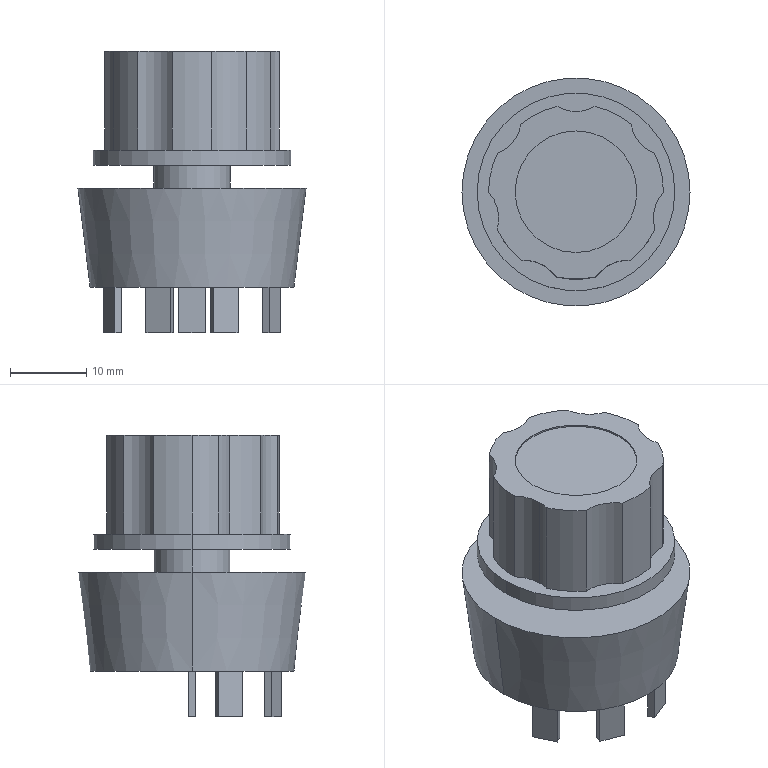Part | SolidWorks | features BaseBody 1 | 1 solid | 55 faces | box 30 x 30 x 37 mm | volume 14720 mm3 | plane 31 | cylinder 22 | cone 2 | commonest cylinder face diameters 10 x10 23 x8 16 x2 26 x2